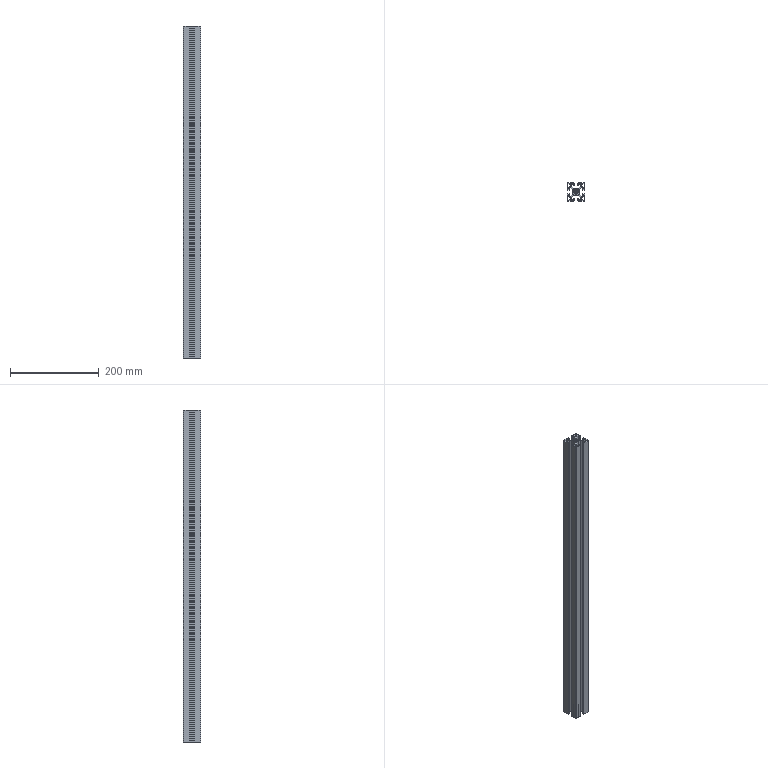Part | SolidWorks | features BaseBody 1, MoveFace 1 | 1 solid | 179 faces | box 40 x 40 x 749 mm | volume 401392 mm3 | plane 130 | cylinder 49 | commonest cylinder face diameters 0.6 x24 2 x8 10 x8 6.8 x5 3 x4